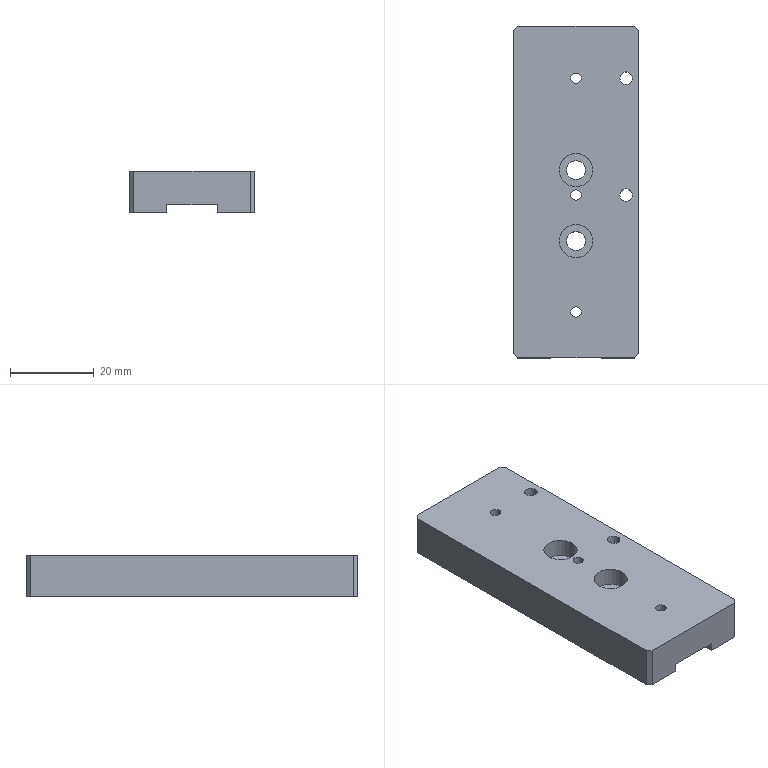Part | STEP file | 11-FG-E01911 | 1 solid | 34 faces | box 30 x 79.5 x 10 mm | volume 21106 mm3 | cylinder 18 | plane 16 | commonest cylinder face diameters 2.5 x6 3 x4 4.5 x4 8 x4
STEP:
#1=CARTESIAN_POINT('',(-4.,5.25,5.6));
#2=VERTEX_POINT('',#1);
#3=CARTESIAN_POINT('',(4.,5.25,5.6));
#4=VERTEX_POINT('',#3);
#5=CARTESIAN_POINT('',(0.,5.25,5.6));
#6=DIRECTION('',(0.,0.,1.));
#7=DIRECTION('',(1.,0.,0.));
#8=AXIS2_PLACEMENT_3D('',#5,#6,#7);
#9=CIRCLE('',#8,4.);
#10=EDGE_CURVE('',#2,#4,#9,.T.);
#11=ORIENTED_EDGE('',*,*,#10,.F.);
#12=CARTESIAN_POINT('',(-4.,5.25,10.));
#13=VERTEX_POINT('',#12);
#14=CARTESIAN_POINT('',(-4.,5.25,10.));
#15=DIRECTION('',(0.,0.,1.));
#16=VECTOR('',#15,1000.);
#17=LINE('',#14,#16);
#18=EDGE_CURVE('',#2,#13,#17,.T.);
#19=ORIENTED_EDGE('',*,*,#18,.T.);
#20=CARTESIAN_POINT('',(4.,5.25,10.));
#21=VERTEX_POINT('',#20);
#22=CARTESIAN_POINT('',(0.,5.25,10.));
#23=DIRECTION('',(0.,0.,1.));
#24=DIRECTION('',(1.,0.,0.));
#25=AXIS2_PLACEMENT_3D('',#22,#23,#24);
#26=CIRCLE('',#25,4.);
#27=EDGE_CURVE('',#13,#21,#26,.T.);
#28=ORIENTED_EDGE('',*,*,#27,.T.);
#29=CARTESIAN_POINT('',(4.,5.25,10.));
#30=DIRECTION('',(0.,0.,1.));
#31=VECTOR('',#30,1000.);
#32=LINE('',#29,#31);
#33=EDGE_CURVE('',#4,#21,#32,.T.);
#34=ORIENTED_EDGE('',*,*,#33,.F.);
#35=EDGE_LOOP('',(#11,#19,#28,#34));
#36=FACE_OUTER_BOUND('',#35,.T.);
#37=CARTESIAN_POINT('',(0.,5.25,10.));
#38=DIRECTION('',(0.,0.,1.));
#39=DIRECTION('',(1.,0.,0.));
#40=AXIS2_PLACEMENT_3D('',#37,#38,#39);
#41=CYLINDRICAL_SURFACE('',#40,4.);
#42=ADVANCED_FACE('',(#36),#41,.F.);
#43=CARTESIAN_POINT('',(2.25,5.25,2.));
#44=VERTEX_POINT('',#43);
#45=CARTESIAN_POINT('',(-2.25,5.25,2.));
#46=VERTEX_POINT('',#45);
#47=CARTESIAN_POINT('',(0.,5.25,2.));
#48=DIRECTION('',(0.,0.,-1.));
#49=DIRECTION('',(-1.,0.,0.));
#50=AXIS2_PLACEMENT_3D('',#47,#48,#49);
#51=CIRCLE('',#50,2.25);
#52=EDGE_CURVE('',#44,#46,#51,.T.);
#53=ORIENTED_EDGE('',*,*,#52,.T.);
#54=CARTESIAN_POINT('',(-2.25,5.25,5.6));
#55=VERTEX_POINT('',#54);
#56=CARTESIAN_POINT('',(-2.25,5.25,10.));
#57=DIRECTION('',(0.,0.,1.));
#58=VECTOR('',#57,1000.);
#59=LINE('',#56,#58);
#60=EDGE_CURVE('',#46,#55,#59,.T.);
#61=ORIENTED_EDGE('',*,*,#60,.T.);
#62=CARTESIAN_POINT('',(2.25,5.25,5.6));
#63=VERTEX_POINT('',#62);
#64=CARTESIAN_POINT('',(0.,5.25,5.6));
#65=DIRECTION('',(0.,0.,1.));
#66=DIRECTION('',(1.,0.,0.));
#67=AXIS2_PLACEMENT_3D('',#64,#65,#66);
#68=CIRCLE('',#67,2.25);
#69=EDGE_CURVE('',#55,#63,#68,.T.);
#70=ORIENTED_EDGE('',*,*,#69,.T.);
#71=CARTESIAN_POINT('',(2.25,5.25,10.));
#72=DIRECTION('',(0.,0.,1.));
#73=VECTOR('',#72,1000.);
#74=LINE('',#71,#73);
#75=EDGE_CURVE('',#44,#63,#74,.T.);
#76=ORIENTED_EDGE('',*,*,#75,.F.);
#77=EDGE_LOOP('',(#53,#61,#70,#76));
#78=FACE_OUTER_BOUND('',#77,.T.);
#79=CARTESIAN_POINT('',(0.,5.25,10.));
#80=DIRECTION('',(0.,0.,1.));
#81=DIRECTION('',(1.,0.,0.));
#82=AXIS2_PLACEMENT_3D('',#79,#80,#81);
#83=CYLINDRICAL_SURFACE('',#82,2.25);
#84=ADVANCED_FACE('',(#78),#83,.F.);
#85=CARTESIAN_POINT('',(-4.,-11.75,5.6));
#86=VERTEX_POINT('',#85);
#87=CARTESIAN_POINT('',(4.,-11.75,5.6));
#88=VERTEX_POINT('',#87);
#89=CARTESIAN_POINT('',(0.,-11.75,5.6));
#90=DIRECTION('',(0.,0.,1.));
#91=DIRECTION('',(1.,0.,0.));
#92=AXIS2_PLACEMENT_3D('',#89,#90,#91);
#93=CIRCLE('',#92,4.);
#94=EDGE_CURVE('',#86,#88,#93,.T.);
#95=ORIENTED_EDGE('',*,*,#94,.F.);
#96=CARTESIAN_POINT('',(-4.,-11.75,10.));
#97=VERTEX_POINT('',#96);
#98=CARTESIAN_POINT('',(-4.,-11.75,10.));
#99=DIRECTION('',(0.,0.,1.));
#100=VECTOR('',#99,1000.);
#101=LINE('',#98,#100);
#102=EDGE_CURVE('',#86,#97,#101,.T.);
#103=ORIENTED_EDGE('',*,*,#102,.T.);
#104=CARTESIAN_POINT('',(4.,-11.75,10.));
#105=VERTEX_POINT('',#104);
#106=CARTESIAN_POINT('',(0.,-11.75,10.));
#107=DIRECTION('',(0.,0.,1.));
#108=DIRECTION('',(1.,0.,0.));
#109=AXIS2_PLACEMENT_3D('',#106,#107,#108);
#110=CIRCLE('',#109,4.);
#111=EDGE_CURVE('',#97,#105,#110,.T.);
#112=ORIENTED_EDGE('',*,*,#111,.T.);
#113=CARTESIAN_POINT('',(4.,-11.75,10.));
#114=DIRECTION('',(0.,0.,1.));
#115=VECTOR('',#114,1000.);
#116=LINE('',#113,#115);
#117=EDGE_CURVE('',#88,#105,#116,.T.);
#118=ORIENTED_EDGE('',*,*,#117,.F.);
#119=EDGE_LOOP('',(#95,#103,#112,#118));
#120=FACE_OUTER_BOUND('',#119,.T.);
#121=CARTESIAN_POINT('',(0.,-11.75,10.));
#122=DIRECTION('',(0.,0.,1.));
#123=DIRECTION('',(1.,0.,0.));
#124=AXIS2_PLACEMENT_3D('',#121,#122,#123);
#125=CYLINDRICAL_SURFACE('',#124,4.);
#126=ADVANCED_FACE('',(#120),#125,.F.);
#127=CARTESIAN_POINT('',(2.25,-11.75,2.));
#128=VERTEX_POINT('',#127);
#129=CARTESIAN_POINT('',(-2.25,-11.75,2.));
#130=VERTEX_POINT('',#129);
#131=CARTESIAN_POINT('',(0.,-11.75,2.));
#132=DIRECTION('',(0.,0.,-1.));
#133=DIRECTION('',(-1.,0.,0.));
#134=AXIS2_PLACEMENT_3D('',#131,#132,#133);
#135=CIRCLE('',#134,2.25);
#136=EDGE_CURVE('',#128,#130,#135,.T.);
#137=ORIENTED_EDGE('',*,*,#136,.T.);
#138=CARTESIAN_POINT('',(-2.25,-11.75,5.6));
#139=VERTEX_POINT('',#138);
#140=CARTESIAN_POINT('',(-2.25,-11.75,10.));
#141=DIRECTION('',(0.,0.,1.));
#142=VECTOR('',#141,1000.);
#143=LINE('',#140,#142);
#144=EDGE_CURVE('',#130,#139,#143,.T.);
#145=ORIENTED_EDGE('',*,*,#144,.T.);
#146=CARTESIAN_POINT('',(2.25,-11.75,5.6));
#147=VERTEX_POINT('',#146);
#148=CARTESIAN_POINT('',(0.,-11.75,5.6));
#149=DIRECTION('',(0.,0.,1.));
#150=DIRECTION('',(1.,0.,0.));
#151=AXIS2_PLACEMENT_3D('',#148,#149,#150);
#152=CIRCLE('',#151,2.25);
#153=EDGE_CURVE('',#139,#147,#152,.T.);
#154=ORIENTED_EDGE('',*,*,#153,.T.);
#155=CARTESIAN_POINT('',(2.25,-11.75,10.));
#156=DIRECTION('',(0.,0.,1.));
#157=VECTOR('',#156,1000.);
#158=LINE('',#155,#157);
#159=EDGE_CURVE('',#128,#147,#158,.T.);
#160=ORIENTED_EDGE('',*,*,#159,.F.);
#161=EDGE_LOOP('',(#137,#145,#154,#160));
#162=FACE_OUTER_BOUND('',#161,.T.);
#163=CARTESIAN_POINT('',(0.,-11.75,10.));
#164=DIRECTION('',(0.,0.,1.));
#165=DIRECTION('',(1.,0.,0.));
#166=AXIS2_PLACEMENT_3D('',#163,#164,#165);
#167=CYLINDRICAL_SURFACE('',#166,2.25);
#168=ADVANCED_FACE('',(#162),#167,.F.);
#169=CARTESIAN_POINT('',(10.5,-0.75,0.));
#170=VERTEX_POINT('',#169);
#171=CARTESIAN_POINT('',(13.5,-0.75,0.));
#172=VERTEX_POINT('',#171);
#173=CARTESIAN_POINT('',(12.,-0.75,0.));
#174=DIRECTION('',(0.,0.,1.));
#175=DIRECTION('',(1.,0.,0.));
#176=AXIS2_PLACEMENT_3D('',#173,#174,#175);
#177=CIRCLE('',#176,1.5);
#178=EDGE_CURVE('',#170,#172,#177,.T.);
#179=ORIENTED_EDGE('',*,*,#178,.F.);
#180=CARTESIAN_POINT('',(10.5,-0.75,10.));
#181=VERTEX_POINT('',#180);
#182=CARTESIAN_POINT('',(10.5,-0.75,10.));
#183=DIRECTION('',(0.,0.,1.));
#184=VECTOR('',#183,1000.);
#185=LINE('',#182,#184);
#186=EDGE_CURVE('',#170,#181,#185,.T.);
#187=ORIENTED_EDGE('',*,*,#186,.T.);
#188=CARTESIAN_POINT('',(13.5,-0.75,10.));
#189=VERTEX_POINT('',#188);
#190=CARTESIAN_POINT('',(12.,-0.75,10.));
#191=DIRECTION('',(0.,0.,1.));
#192=DIRECTION('',(1.,0.,0.));
#193=AXIS2_PLACEMENT_3D('',#190,#191,#192);
#194=CIRCLE('',#193,1.5);
#195=EDGE_CURVE('',#181,#189,#194,.T.);
#196=ORIENTED_EDGE('',*,*,#195,.T.);
#197=CARTESIAN_POINT('',(13.5,-0.75,10.));
#198=DIRECTION('',(0.,0.,1.));
#199=VECTOR('',#198,1000.);
#200=LINE('',#197,#199);
#201=EDGE_CURVE('',#172,#189,#200,.T.);
#202=ORIENTED_EDGE('',*,*,#201,.F.);
#203=EDGE_LOOP('',(#179,#187,#196,#202));
#204=FACE_OUTER_BOUND('',#203,.T.);
#205=CARTESIAN_POINT('',(12.,-0.75,10.));
#206=DIRECTION('',(0.,0.,1.));
#207=DIRECTION('',(1.,0.,0.));
#208=AXIS2_PLACEMENT_3D('',#205,#206,#207);
#209=CYLINDRICAL_SURFACE('',#208,1.5);
#210=ADVANCED_FACE('',(#204),#209,.F.);
#211=CARTESIAN_POINT('',(10.5,27.25,0.));
#212=VERTEX_POINT('',#211);
#213=CARTESIAN_POINT('',(13.5,27.25,0.));
#214=VERTEX_POINT('',#213);
#215=CARTESIAN_POINT('',(12.,27.25,0.));
#216=DIRECTION('',(0.,0.,1.));
#217=DIRECTION('',(1.,0.,0.));
#218=AXIS2_PLACEMENT_3D('',#215,#216,#217);
#219=CIRCLE('',#218,1.5);
#220=EDGE_CURVE('',#212,#214,#219,.T.);
#221=ORIENTED_EDGE('',*,*,#220,.F.);
#222=CARTESIAN_POINT('',(10.5,27.25,10.));
#223=VERTEX_POINT('',#222);
#224=CARTESIAN_POINT('',(10.5,27.25,10.));
#225=DIRECTION('',(0.,0.,1.));
#226=VECTOR('',#225,1000.);
#227=LINE('',#224,#226);
#228=EDGE_CURVE('',#212,#223,#227,.T.);
#229=ORIENTED_EDGE('',*,*,#228,.T.);
#230=CARTESIAN_POINT('',(13.5,27.25,10.));
#231=VERTEX_POINT('',#230);
#232=CARTESIAN_POINT('',(12.,27.25,10.));
#233=DIRECTION('',(0.,0.,1.));
#234=DIRECTION('',(1.,0.,0.));
#235=AXIS2_PLACEMENT_3D('',#232,#233,#234);
#236=CIRCLE('',#235,1.5);
#237=EDGE_CURVE('',#223,#231,#236,.T.);
#238=ORIENTED_EDGE('',*,*,#237,.T.);
#239=CARTESIAN_POINT('',(13.5,27.25,10.));
#240=DIRECTION('',(0.,0.,1.));
#241=VECTOR('',#240,1000.);
#242=LINE('',#239,#241);
#243=EDGE_CURVE('',#214,#231,#242,.T.);
#244=ORIENTED_EDGE('',*,*,#243,.F.);
#245=EDGE_LOOP('',(#221,#229,#238,#244));
#246=FACE_OUTER_BOUND('',#245,.T.);
#247=CARTESIAN_POINT('',(12.,27.25,10.));
#248=DIRECTION('',(0.,0.,1.));
#249=DIRECTION('',(1.,0.,0.));
#250=AXIS2_PLACEMENT_3D('',#247,#248,#249);
#251=CYLINDRICAL_SURFACE('',#250,1.5);
#252=ADVANCED_FACE('',(#246),#251,.F.);
#253=CARTESIAN_POINT('',(1.25,-28.75,2.));
#254=VERTEX_POINT('',#253);
#255=CARTESIAN_POINT('',(-1.25,-28.75,2.));
#256=VERTEX_POINT('',#255);
#257=CARTESIAN_POINT('',(0.,-28.75,2.));
#258=DIRECTION('',(0.,0.,-1.));
#259=DIRECTION('',(-1.,0.,0.));
#260=AXIS2_PLACEMENT_3D('',#257,#258,#259);
#261=CIRCLE('',#260,1.25);
#262=EDGE_CURVE('',#254,#256,#261,.T.);
#263=ORIENTED_EDGE('',*,*,#262,.T.);
#264=CARTESIAN_POINT('',(-1.25,-28.75,10.));
#265=VERTEX_POINT('',#264);
#266=CARTESIAN_POINT('',(-1.25,-28.75,10.));
#267=DIRECTION('',(0.,0.,1.));
#268=VECTOR('',#267,1000.);
#269=LINE('',#266,#268);
#270=EDGE_CURVE('',#256,#265,#269,.T.);
#271=ORIENTED_EDGE('',*,*,#270,.T.);
#272=CARTESIAN_POINT('',(1.25,-28.75,10.));
#273=VERTEX_POINT('',#272);
#274=CARTESIAN_POINT('',(0.,-28.75,10.));
#275=DIRECTION('',(0.,0.,1.));
#276=DIRECTION('',(1.,0.,0.));
#277=AXIS2_PLACEMENT_3D('',#274,#275,#276);
#278=CIRCLE('',#277,1.25);
#279=EDGE_CURVE('',#265,#273,#278,.T.);
#280=ORIENTED_EDGE('',*,*,#279,.T.);
#281=CARTESIAN_POINT('',(1.25,-28.75,10.));
#282=DIRECTION('',(0.,0.,1.));
#283=VECTOR('',#282,1000.);
#284=LINE('',#281,#283);
#285=EDGE_CURVE('',#254,#273,#284,.T.);
#286=ORIENTED_EDGE('',*,*,#285,.F.);
#287=EDGE_LOOP('',(#263,#271,#280,#286));
#288=FACE_OUTER_BOUND('',#287,.T.);
#289=CARTESIAN_POINT('',(0.,-28.75,10.));
#290=DIRECTION('',(0.,0.,1.));
#291=DIRECTION('',(1.,0.,0.));
#292=AXIS2_PLACEMENT_3D('',#289,#290,#291);
#293=CYLINDRICAL_SURFACE('',#292,1.25);
#294=ADVANCED_FACE('',(#288),#293,.F.);
#295=CARTESIAN_POINT('',(1.25,-0.75,2.));
#296=VERTEX_POINT('',#295);
#297=CARTESIAN_POINT('',(-1.25,-0.75,2.));
#298=VERTEX_POINT('',#297);
#299=CARTESIAN_POINT('',(0.,-0.75,2.));
#300=DIRECTION('',(0.,0.,-1.));
#301=DIRECTION('',(-1.,0.,0.));
#302=AXIS2_PLACEMENT_3D('',#299,#300,#301);
#303=CIRCLE('',#302,1.25);
#304=EDGE_CURVE('',#296,#298,#303,.T.);
#305=ORIENTED_EDGE('',*,*,#304,.T.);
#306=CARTESIAN_POINT('',(-1.25,-0.75,10.));
#307=VERTEX_POINT('',#306);
#308=CARTESIAN_POINT('',(-1.25,-0.75,10.));
#309=DIRECTION('',(0.,0.,1.));
#310=VECTOR('',#309,1000.);
#311=LINE('',#308,#310);
#312=EDGE_CURVE('',#298,#307,#311,.T.);
#313=ORIENTED_EDGE('',*,*,#312,.T.);
#314=CARTESIAN_POINT('',(1.25,-0.75,10.));
#315=VERTEX_POINT('',#314);
#316=CARTESIAN_POINT('',(0.,-0.75,10.));
#317=DIRECTION('',(0.,0.,1.));
#318=DIRECTION('',(1.,0.,0.));
#319=AXIS2_PLACEMENT_3D('',#316,#317,#318);
#320=CIRCLE('',#319,1.25);
#321=EDGE_CURVE('',#307,#315,#320,.T.);
#322=ORIENTED_EDGE('',*,*,#321,.T.);
#323=CARTESIAN_POINT('',(1.25,-0.75,10.));
#324=DIRECTION('',(0.,0.,1.));
#325=VECTOR('',#324,1000.);
#326=LINE('',#323,#325);
#327=EDGE_CURVE('',#296,#315,#326,.T.);
#328=ORIENTED_EDGE('',*,*,#327,.F.);
#329=EDGE_LOOP('',(#305,#313,#322,#328));
#330=FACE_OUTER_BOUND('',#329,.T.);
#331=CARTESIAN_POINT('',(0.,-0.75,10.));
#332=DIRECTION('',(0.,0.,1.));
#333=DIRECTION('',(1.,0.,0.));
#334=AXIS2_PLACEMENT_3D('',#331,#332,#333);
#335=CYLINDRICAL_SURFACE('',#334,1.25);
#336=ADVANCED_FACE('',(#330),#335,.F.);
#337=CARTESIAN_POINT('',(1.25,27.25,2.));
#338=VERTEX_POINT('',#337);
#339=CARTESIAN_POINT('',(-1.25,27.25,2.));
#340=VERTEX_POINT('',#339);
#341=CARTESIAN_POINT('',(0.,27.25,2.));
#342=DIRECTION('',(0.,0.,-1.));
#343=DIRECTION('',(-1.,0.,0.));
#344=AXIS2_PLACEMENT_3D('',#341,#342,#343);
#345=CIRCLE('',#344,1.25);
#346=EDGE_CURVE('',#338,#340,#345,.T.);
#347=ORIENTED_EDGE('',*,*,#346,.T.);
#348=CARTESIAN_POINT('',(-1.25,27.25,10.));
#349=VERTEX_POINT('',#348);
#350=CARTESIAN_POINT('',(-1.25,27.25,10.));
#351=DIRECTION('',(0.,0.,1.));
#352=VECTOR('',#351,1000.);
#353=LINE('',#350,#352);
#354=EDGE_CURVE('',#340,#349,#353,.T.);
#355=ORIENTED_EDGE('',*,*,#354,.T.);
#356=CARTESIAN_POINT('',(1.25,27.25,10.));
#357=VERTEX_POINT('',#356);
#358=CARTESIAN_POINT('',(0.,27.25,10.));
#359=DIRECTION('',(0.,0.,1.));
#360=DIRECTION('',(1.,0.,0.));
#361=AXIS2_PLACEMENT_3D('',#358,#359,#360);
#362=CIRCLE('',#361,1.25);
#363=EDGE_CURVE('',#349,#357,#362,.T.);
#364=ORIENTED_EDGE('',*,*,#363,.T.);
#365=CARTESIAN_POINT('',(1.25,27.25,10.));
#366=DIRECTION('',(0.,0.,1.));
#367=VECTOR('',#366,1000.);
#368=LINE('',#365,#367);
#369=EDGE_CURVE('',#338,#357,#368,.T.);
#370=ORIENTED_EDGE('',*,*,#369,.F.);
#371=EDGE_LOOP('',(#347,#355,#364,#370));
#372=FACE_OUTER_BOUND('',#371,.T.);
#373=CARTESIAN_POINT('',(0.,27.25,10.));
#374=DIRECTION('',(0.,0.,1.));
#375=DIRECTION('',(1.,0.,0.));
#376=AXIS2_PLACEMENT_3D('',#373,#374,#375);
#377=CYLINDRICAL_SURFACE('',#376,1.25);
#378=ADVANCED_FACE('',(#372),#377,.F.);
#379=CARTESIAN_POINT('',(12.,-0.75,0.));
#380=DIRECTION('',(0.,0.,1.));
#381=DIRECTION('',(1.,0.,0.));
#382=AXIS2_PLACEMENT_3D('',#379,#380,#381);
#383=CIRCLE('',#382,1.5);
#384=EDGE_CURVE('',#172,#170,#383,.T.);
#385=ORIENTED_EDGE('',*,*,#384,.T.);
#386=ORIENTED_EDGE('',*,*,#178,.T.);
#387=EDGE_LOOP('',(#385,#386));
#388=FACE_BOUND('',#387,.T.);
#389=CARTESIAN_POINT('',(12.,27.25,0.));
#390=DIRECTION('',(0.,0.,1.));
#391=DIRECTION('',(1.,0.,0.));
#392=AXIS2_PLACEMENT_3D('',#389,#390,#391);
#393=CIRCLE('',#392,1.5);
#394=EDGE_CURVE('',#214,#212,#393,.T.);
#395=ORIENTED_EDGE('',*,*,#394,.T.);
#396=ORIENTED_EDGE('',*,*,#220,.T.);
#397=EDGE_LOOP('',(#395,#396));
#398=FACE_BOUND('',#397,.T.);
#399=CARTESIAN_POINT('',(15.,-38.75,0.));
#400=VERTEX_POINT('',#399);
#401=CARTESIAN_POINT('',(15.,38.75,0.));
#402=VERTEX_POINT('',#401);
#403=CARTESIAN_POINT('',(15.,-39.75,0.));
#404=DIRECTION('',(0.,1.,0.));
#405=VECTOR('',#404,1000.);
#406=LINE('',#403,#405);
#407=EDGE_CURVE('',#400,#402,#406,.T.);
#408=ORIENTED_EDGE('',*,*,#407,.F.);
#409=CARTESIAN_POINT('',(14.,-39.75,0.));
#410=VERTEX_POINT('',#409);
#411=CARTESIAN_POINT('',(26.875,-26.875,0.));
#412=DIRECTION('',(-0.7071,-0.7071,0.));
#413=VECTOR('',#412,1000.);
#414=LINE('',#411,#413);
#415=EDGE_CURVE('',#400,#410,#414,.T.);
#416=ORIENTED_EDGE('',*,*,#415,.T.);
#417=CARTESIAN_POINT('',(6.,-39.75,0.));
#418=VERTEX_POINT('',#417);
#419=CARTESIAN_POINT('',(-15.,-39.75,0.));
#420=DIRECTION('',(1.,0.,0.));
#421=VECTOR('',#420,1000.);
#422=LINE('',#419,#421);
#423=EDGE_CURVE('',#418,#410,#422,.T.);
#424=ORIENTED_EDGE('',*,*,#423,.F.);
#425=CARTESIAN_POINT('',(6.,39.75,0.));
#426=VERTEX_POINT('',#425);
#427=CARTESIAN_POINT('',(6.,-39.75,0.));
#428=DIRECTION('',(0.,-1.,0.));
#429=VECTOR('',#428,1000.);
#430=LINE('',#427,#429);
#431=EDGE_CURVE('',#426,#418,#430,.T.);
#432=ORIENTED_EDGE('',*,*,#431,.F.);
#433=CARTESIAN_POINT('',(14.,39.75,0.));
#434=VERTEX_POINT('',#433);
#435=CARTESIAN_POINT('',(-15.,39.75,0.));
#436=DIRECTION('',(-1.,0.,0.));
#437=VECTOR('',#436,1000.);
#438=LINE('',#435,#437);
#439=EDGE_CURVE('',#434,#426,#438,.T.);
#440=ORIENTED_EDGE('',*,*,#439,.F.);
#441=CARTESIAN_POINT('',(26.875,26.875,0.));
#442=DIRECTION('',(0.7071,-0.7071,0.));
#443=VECTOR('',#442,1000.);
#444=LINE('',#441,#443);
#445=EDGE_CURVE('',#434,#402,#444,.T.);
#446=ORIENTED_EDGE('',*,*,#445,.T.);
#447=EDGE_LOOP('',(#408,#416,#424,#432,#440,#446));
#448=FACE_OUTER_BOUND('',#447,.T.);
#449=CARTESIAN_POINT('',(0.,0.,0.));
#450=DIRECTION('',(0.,0.,-1.));
#451=DIRECTION('',(-1.,0.,0.));
#452=AXIS2_PLACEMENT_3D('',#449,#450,#451);
#453=PLANE('',#452);
#454=ADVANCED_FACE('',(#388,#398,#448),#453,.T.);
#455=CARTESIAN_POINT('',(15.,-38.75,10.));
#456=VERTEX_POINT('',#455);
#457=CARTESIAN_POINT('',(15.,38.75,10.));
#458=VERTEX_POINT('',#457);
#459=CARTESIAN_POINT('',(15.,-39.75,10.));
#460=DIRECTION('',(0.,1.,0.));
#461=VECTOR('',#460,1000.);
#462=LINE('',#459,#461);
#463=EDGE_CURVE('',#456,#458,#462,.T.);
#464=ORIENTED_EDGE('',*,*,#463,.F.);
#465=CARTESIAN_POINT('',(15.,-38.75,10.));
#466=DIRECTION('',(0.,0.,-1.));
#467=VECTOR('',#466,1000.);
#468=LINE('',#465,#467);
#469=EDGE_CURVE('',#456,#400,#468,.T.);
#470=ORIENTED_EDGE('',*,*,#469,.T.);
#471=ORIENTED_EDGE('',*,*,#407,.T.);
#472=CARTESIAN_POINT('',(15.,38.75,10.));
#473=DIRECTION('',(0.,0.,1.));
#474=VECTOR('',#473,1000.);
#475=LINE('',#472,#474);
#476=EDGE_CURVE('',#402,#458,#475,.T.);
#477=ORIENTED_EDGE('',*,*,#476,.T.);
#478=EDGE_LOOP('',(#464,#470,#471,#477));
#479=FACE_OUTER_BOUND('',#478,.T.);
#480=CARTESIAN_POINT('',(15.,-39.75,10.));
#481=DIRECTION('',(-1.,0.,0.));
#482=DIRECTION('',(0.,0.,1.));
#483=AXIS2_PLACEMENT_3D('',#480,#481,#482);
#484=PLANE('',#483);
#485=ADVANCED_FACE('',(#479),#484,.F.);
#486=CARTESIAN_POINT('',(14.,39.75,10.));
#487=VERTEX_POINT('',#486);
#488=CARTESIAN_POINT('',(-14.,39.75,10.));
#489=VERTEX_POINT('',#488);
#490=CARTESIAN_POINT('',(-15.,39.75,10.));
#491=DIRECTION('',(-1.,0.,0.));
#492=VECTOR('',#491,1000.);
#493=LINE('',#490,#492);
#494=EDGE_CURVE('',#487,#489,#493,.T.);
#495=ORIENTED_EDGE('',*,*,#494,.F.);
#496=CARTESIAN_POINT('',(14.,39.75,10.));
#497=DIRECTION('',(0.,0.,-1.));
#498=VECTOR('',#497,1000.);
#499=LINE('',#496,#498);
#500=EDGE_CURVE('',#487,#434,#499,.T.);
#501=ORIENTED_EDGE('',*,*,#500,.T.);
#502=ORIENTED_EDGE('',*,*,#439,.T.);
#503=CARTESIAN_POINT('',(6.,39.75,2.));
#504=VERTEX_POINT('',#503);
#505=CARTESIAN_POINT('',(6.,39.75,2.));
#506=DIRECTION('',(0.,0.,-1.));
#507=VECTOR('',#506,1000.);
#508=LINE('',#505,#507);
#509=EDGE_CURVE('',#504,#426,#508,.T.);
#510=ORIENTED_EDGE('',*,*,#509,.F.);
#511=CARTESIAN_POINT('',(-6.,39.75,2.));
#512=VERTEX_POINT('',#511);
#513=CARTESIAN_POINT('',(-6.,39.75,2.));
#514=DIRECTION('',(1.,0.,0.));
#515=VECTOR('',#514,1000.);
#516=LINE('',#513,#515);
#517=EDGE_CURVE('',#512,#504,#516,.T.);
#518=ORIENTED_EDGE('',*,*,#517,.F.);
#519=CARTESIAN_POINT('',(-6.,39.75,0.));
#520=VERTEX_POINT('',#519);
#521=CARTESIAN_POINT('',(-6.,39.75,2.));
#522=DIRECTION('',(0.,0.,-1.));
#523=VECTOR('',#522,1000.);
#524=LINE('',#521,#523);
#525=EDGE_CURVE('',#512,#520,#524,.T.);
#526=ORIENTED_EDGE('',*,*,#525,.T.);
#527=CARTESIAN_POINT('',(-14.,39.75,0.));
#528=VERTEX_POINT('',#527);
#529=CARTESIAN_POINT('',(-15.,39.75,0.));
#530=DIRECTION('',(-1.,0.,0.));
#531=VECTOR('',#530,1000.);
#532=LINE('',#529,#531);
#533=EDGE_CURVE('',#520,#528,#532,.T.);
#534=ORIENTED_EDGE('',*,*,#533,.T.);
#535=CARTESIAN_POINT('',(-14.,39.75,10.));
#536=DIRECTION('',(0.,0.,1.));
#537=VECTOR('',#536,1000.);
#538=LINE('',#535,#537);
#539=EDGE_CURVE('',#528,#489,#538,.T.);
#540=ORIENTED_EDGE('',*,*,#539,.T.);
#541=EDGE_LOOP('',(#495,#501,#502,#510,#518,#526,#534,#540));
#542=FACE_OUTER_BOUND('',#541,.T.);
#543=CARTESIAN_POINT('',(-15.,39.75,10.));
#544=DIRECTION('',(0.,-1.,0.));
#545=DIRECTION('',(0.,0.,-1.));
#546=AXIS2_PLACEMENT_3D('',#543,#544,#545);
#547=PLANE('',#546);
#548=ADVANCED_FACE('',(#542),#547,.F.);
#549=CARTESIAN_POINT('',(-15.,38.75,0.));
#550=VERTEX_POINT('',#549);
#551=CARTESIAN_POINT('',(-15.,-38.75,0.));
#552=VERTEX_POINT('',#551);
#553=CARTESIAN_POINT('',(-15.,-39.75,0.));
#554=DIRECTION('',(0.,-1.,0.));
#555=VECTOR('',#554,1000.);
#556=LINE('',#553,#555);
#557=EDGE_CURVE('',#550,#552,#556,.T.);
#558=ORIENTED_EDGE('',*,*,#557,.T.);
#559=CARTESIAN_POINT('',(-15.,-38.75,10.));
#560=VERTEX_POINT('',#559);
#561=CARTESIAN_POINT('',(-15.,-38.75,10.));
#562=DIRECTION('',(0.,0.,1.));
#563=VECTOR('',#562,1000.);
#564=LINE('',#561,#563);
#565=EDGE_CURVE('',#552,#560,#564,.T.);
#566=ORIENTED_EDGE('',*,*,#565,.T.);
#567=CARTESIAN_POINT('',(-15.,38.75,10.));
#568=VERTEX_POINT('',#567);
#569=CARTESIAN_POINT('',(-15.,-39.75,10.));
#570=DIRECTION('',(0.,-1.,0.));
#571=VECTOR('',#570,1000.);
#572=LINE('',#569,#571);
#573=EDGE_CURVE('',#568,#560,#572,.T.);
#574=ORIENTED_EDGE('',*,*,#573,.F.);
#575=CARTESIAN_POINT('',(-15.,38.75,10.));
#576=DIRECTION('',(0.,0.,-1.));
#577=VECTOR('',#576,1000.);
#578=LINE('',#575,#577);
#579=EDGE_CURVE('',#568,#550,#578,.T.);
#580=ORIENTED_EDGE('',*,*,#579,.T.);
#581=EDGE_LOOP('',(#558,#566,#574,#580));
#582=FACE_OUTER_BOUND('',#581,.T.);
#583=CARTESIAN_POINT('',(-15.,-39.75,10.));
#584=DIRECTION('',(1.,0.,0.));
#585=DIRECTION('',(0.,0.,-1.));
#586=AXIS2_PLACEMENT_3D('',#583,#584,#585);
#587=PLANE('',#586);
#588=ADVANCED_FACE('',(#582),#587,.F.);
#589=CARTESIAN_POINT('',(-14.,-39.75,10.));
#590=VERTEX_POINT('',#589);
#591=CARTESIAN_POINT('',(14.,-39.75,10.));
#592=VERTEX_POINT('',#591);
#593=CARTESIAN_POINT('',(-15.,-39.75,10.));
#594=DIRECTION('',(1.,0.,0.));
#595=VECTOR('',#594,1000.);
#596=LINE('',#593,#595);
#597=EDGE_CURVE('',#590,#592,#596,.T.);
#598=ORIENTED_EDGE('',*,*,#597,.F.);
#599=CARTESIAN_POINT('',(-14.,-39.75,0.));
#600=VERTEX_POINT('',#599);
#601=CARTESIAN_POINT('',(-14.,-39.75,10.));
#602=DIRECTION('',(0.,0.,-1.));
#603=VECTOR('',#602,1000.);
#604=LINE('',#601,#603);
#605=EDGE_CURVE('',#590,#600,#604,.T.);
#606=ORIENTED_EDGE('',*,*,#605,.T.);
#607=CARTESIAN_POINT('',(-6.,-39.75,0.));
#608=VERTEX_POINT('',#607);
#609=CARTESIAN_POINT('',(-15.,-39.75,0.));
#610=DIRECTION('',(1.,0.,0.));
#611=VECTOR('',#610,1000.);
#612=LINE('',#609,#611);
#613=EDGE_CURVE('',#600,#608,#612,.T.);
#614=ORIENTED_EDGE('',*,*,#613,.T.);
#615=CARTESIAN_POINT('',(-6.,-39.75,2.));
#616=VERTEX_POINT('',#615);
#617=CARTESIAN_POINT('',(-6.,-39.75,2.));
#618=DIRECTION('',(0.,0.,-1.));
#619=VECTOR('',#618,1000.);
#620=LINE('',#617,#619);
#621=EDGE_CURVE('',#616,#608,#620,.T.);
#622=ORIENTED_EDGE('',*,*,#621,.F.);
#623=CARTESIAN_POINT('',(6.,-39.75,2.));
#624=VERTEX_POINT('',#623);
#625=CARTESIAN_POINT('',(-6.,-39.75,2.));
#626=DIRECTION('',(-1.,0.,0.));
#627=VECTOR('',#626,1000.);
#628=LINE('',#625,#627);
#629=EDGE_CURVE('',#624,#616,#628,.T.);
#630=ORIENTED_EDGE('',*,*,#629,.F.);
#631=CARTESIAN_POINT('',(6.,-39.75,2.));
#632=DIRECTION('',(0.,0.,-1.));
#633=VECTOR('',#632,1000.);
#634=LINE('',#631,#633);
#635=EDGE_CURVE('',#624,#418,#634,.T.);
#636=ORIENTED_EDGE('',*,*,#635,.T.);
#637=ORIENTED_EDGE('',*,*,#423,.T.);
#638=CARTESIAN_POINT('',(14.,-39.75,10.));
#639=DIRECTION('',(0.,0.,1.));
#640=VECTOR('',#639,1000.);
#641=LINE('',#638,#640);
#642=EDGE_CURVE('',#410,#592,#641,.T.);
#643=ORIENTED_EDGE('',*,*,#642,.T.);
#644=EDGE_LOOP('',(#598,#606,#614,#622,#630,#636,#637,#643));
#645=FACE_OUTER_BOUND('',#644,.T.);
#646=CARTESIAN_POINT('',(-15.,-39.75,10.));
#647=DIRECTION('',(0.,1.,0.));
#648=DIRECTION('',(0.,0.,1.));
#649=AXIS2_PLACEMENT_3D('',#646,#647,#648);
#650=PLANE('',#649);
#651=ADVANCED_FACE('',(#645),#650,.F.);
#652=CARTESIAN_POINT('',(0.,5.25,10.));
#653=DIRECTION('',(0.,0.,1.));
#654=DIRECTION('',(1.,0.,0.));
#655=AXIS2_PLACEMENT_3D('',#652,#653,#654);
#656=CIRCLE('',#655,4.);
#657=EDGE_CURVE('',#21,#13,#656,.T.);
#658=ORIENTED_EDGE('',*,*,#657,.F.);
#659=ORIENTED_EDGE('',*,*,#27,.F.);
#660=EDGE_LOOP('',(#658,#659));
#661=FACE_BOUND('',#660,.T.);
#662=CARTESIAN_POINT('',(0.,-11.75,10.));
#663=DIRECTION('',(0.,0.,1.));
#664=DIRECTION('',(1.,0.,0.));
#665=AXIS2_PLACEMENT_3D('',#662,#663,#664);
#666=CIRCLE('',#665,4.);
#667=EDGE_CURVE('',#105,#97,#666,.T.);
#668=ORIENTED_EDGE('',*,*,#667,.F.);
#669=ORIENTED_EDGE('',*,*,#111,.F.);
#670=EDGE_LOOP('',(#668,#669));
#671=FACE_BOUND('',#670,.T.);
#672=CARTESIAN_POINT('',(12.,-0.75,10.));
#673=DIRECTION('',(0.,0.,1.));
#674=DIRECTION('',(1.,0.,0.));
#675=AXIS2_PLACEMENT_3D('',#672,#673,#674);
#676=CIRCLE('',#675,1.5);
#677=EDGE_CURVE('',#189,#181,#676,.T.);
#678=ORIENTED_EDGE('',*,*,#677,.F.);
#679=ORIENTED_EDGE('',*,*,#195,.F.);
#680=EDGE_LOOP('',(#678,#679));
#681=FACE_BOUND('',#680,.T.);
#682=CARTESIAN_POINT('',(12.,27.25,10.));
#683=DIRECTION('',(0.,0.,1.));
#684=DIRECTION('',(1.,0.,0.));
#685=AXIS2_PLACEMENT_3D('',#682,#683,#684);
#686=CIRCLE('',#685,1.5);
#687=EDGE_CURVE('',#231,#223,#686,.T.);
#688=ORIENTED_EDGE('',*,*,#687,.F.);
#689=ORIENTED_EDGE('',*,*,#237,.F.);
#690=EDGE_LOOP('',(#688,#689));
#691=FACE_BOUND('',#690,.T.);
#692=CARTESIAN_POINT('',(0.,-28.75,10.));
#693=DIRECTION('',(0.,0.,1.));
#694=DIRECTION('',(1.,0.,0.));
#695=AXIS2_PLACEMENT_3D('',#692,#693,#694);
#696=CIRCLE('',#695,1.25);
#697=EDGE_CURVE('',#273,#265,#696,.T.);
#698=ORIENTED_EDGE('',*,*,#697,.F.);
#699=ORIENTED_EDGE('',*,*,#279,.F.);
#700=EDGE_LOOP('',(#698,#699));
#701=FACE_BOUND('',#700,.T.);
#702=CARTESIAN_POINT('',(0.,-0.75,10.));
#703=DIRECTION('',(0.,0.,1.));
#704=DIRECTION('',(1.,0.,0.));
#705=AXIS2_PLACEMENT_3D('',#702,#703,#704);
#706=CIRCLE('',#705,1.25);
#707=EDGE_CURVE('',#315,#307,#706,.T.);
#708=ORIENTED_EDGE('',*,*,#707,.F.);
#709=ORIENTED_EDGE('',*,*,#321,.F.);
#710=EDGE_LOOP('',(#708,#709));
#711=FACE_BOUND('',#710,.T.);
#712=CARTESIAN_POINT('',(0.,27.25,10.));
#713=DIRECTION('',(0.,0.,1.));
#714=DIRECTION('',(1.,0.,0.));
#715=AXIS2_PLACEMENT_3D('',#712,#713,#714);
#716=CIRCLE('',#715,1.25);
#717=EDGE_CURVE('',#357,#349,#716,.T.);
#718=ORIENTED_EDGE('',*,*,#717,.F.);
#719=ORIENTED_EDGE('',*,*,#363,.F.);
#720=EDGE_LOOP('',(#718,#719));
#721=FACE_BOUND('',#720,.T.);
#722=ORIENTED_EDGE('',*,*,#573,.T.);
#723=CARTESIAN_POINT('',(-14.,-39.75,10.));
#724=DIRECTION('',(0.7071,-0.7071,0.));
#725=VECTOR('',#724,1000.);
#726=LINE('',#723,#725);
#727=EDGE_CURVE('',#560,#590,#726,.T.);
#728=ORIENTED_EDGE('',*,*,#727,.T.);
#729=ORIENTED_EDGE('',*,*,#597,.T.);
#730=CARTESIAN_POINT('',(15.,-38.75,10.));
#731=DIRECTION('',(0.7071,0.7071,0.));
#732=VECTOR('',#731,1000.);
#733=LINE('',#730,#732);
#734=EDGE_CURVE('',#592,#456,#733,.T.);
#735=ORIENTED_EDGE('',*,*,#734,.T.);
#736=ORIENTED_EDGE('',*,*,#463,.T.);
#737=CARTESIAN_POINT('',(14.,39.75,10.));
#738=DIRECTION('',(-0.7071,0.7071,0.));
#739=VECTOR('',#738,1000.);
#740=LINE('',#737,#739);
#741=EDGE_CURVE('',#458,#487,#740,.T.);
#742=ORIENTED_EDGE('',*,*,#741,.T.);
#743=ORIENTED_EDGE('',*,*,#494,.T.);
#744=CARTESIAN_POINT('',(-15.,38.75,10.));
#745=DIRECTION('',(-0.7071,-0.7071,0.));
#746=VECTOR('',#745,1000.);
#747=LINE('',#744,#746);
#748=EDGE_CURVE('',#489,#568,#747,.T.);
#749=ORIENTED_EDGE('',*,*,#748,.T.);
#750=EDGE_LOOP('',(#722,#728,#729,#735,#736,#742,#743,#749));
#751=FACE_OUTER_BOUND('',#750,.T.);
#752=CARTESIAN_POINT('',(0.,0.,10.));
#753=DIRECTION('',(0.,0.,-1.));
#754=DIRECTION('',(-1.,0.,0.));
#755=AXIS2_PLACEMENT_3D('',#752,#753,#754);
#756=PLANE('',#755);
#757=ADVANCED_FACE('',(#661,#671,#681,#691,#701,#711,#721,#751),#756,.F.);
#758=ORIENTED_EDGE('',*,*,#613,.F.);
#759=CARTESIAN_POINT('',(-26.875,-26.875,0.));
#760=DIRECTION('',(-0.7071,0.7071,0.));
#761=VECTOR('',#760,1000.);
#762=LINE('',#759,#761);
#763=EDGE_CURVE('',#600,#552,#762,.T.);
#764=ORIENTED_EDGE('',*,*,#763,.T.);
#765=ORIENTED_EDGE('',*,*,#557,.F.);
#766=CARTESIAN_POINT('',(-26.875,26.875,0.));
#767=DIRECTION('',(0.7071,0.7071,0.));
#768=VECTOR('',#767,1000.);
#769=LINE('',#766,#768);
#770=EDGE_CURVE('',#550,#528,#769,.T.);
#771=ORIENTED_EDGE('',*,*,#770,.T.);
#772=ORIENTED_EDGE('',*,*,#533,.F.);
#773=CARTESIAN_POINT('',(-6.,-39.75,0.));
#774=DIRECTION('',(0.,1.,0.));
#775=VECTOR('',#774,1000.);
#776=LINE('',#773,#775);
#777=EDGE_CURVE('',#608,#520,#776,.T.);
#778=ORIENTED_EDGE('',*,*,#777,.F.);
#779=EDGE_LOOP('',(#758,#764,#765,#771,#772,#778));
#780=FACE_OUTER_BOUND('',#779,.T.);
#781=CARTESIAN_POINT('',(0.,0.,0.));
#782=DIRECTION('',(0.,0.,-1.));
#783=DIRECTION('',(-1.,0.,0.));
#784=AXIS2_PLACEMENT_3D('',#781,#782,#783);
#785=PLANE('',#784);
#786=ADVANCED_FACE('',(#780),#785,.T.);
#787=ORIENTED_EDGE('',*,*,#431,.T.);
#788=ORIENTED_EDGE('',*,*,#635,.F.);
#789=CARTESIAN_POINT('',(6.,-39.75,2.));
#790=DIRECTION('',(0.,-1.,0.));
#791=VECTOR('',#790,1000.);
#792=LINE('',#789,#791);
#793=EDGE_CURVE('',#504,#624,#792,.T.);
#794=ORIENTED_EDGE('',*,*,#793,.F.);
#795=ORIENTED_EDGE('',*,*,#509,.T.);
#796=EDGE_LOOP('',(#787,#788,#794,#795));
#797=FACE_OUTER_BOUND('',#796,.T.);
#798=CARTESIAN_POINT('',(6.,-39.75,2.));
#799=DIRECTION('',(1.,0.,0.));
#800=DIRECTION('',(0.,0.,-1.));
#801=AXIS2_PLACEMENT_3D('',#798,#799,#800);
#802=PLANE('',#801);
#803=ADVANCED_FACE('',(#797),#802,.F.);
#804=ORIENTED_EDGE('',*,*,#777,.T.);
#805=ORIENTED_EDGE('',*,*,#525,.F.);
#806=CARTESIAN_POINT('',(-6.,-39.75,2.));
#807=DIRECTION('',(0.,1.,0.));
#808=VECTOR('',#807,1000.);
#809=LINE('',#806,#808);
#810=EDGE_CURVE('',#616,#512,#809,.T.);
#811=ORIENTED_EDGE('',*,*,#810,.F.);
#812=ORIENTED_EDGE('',*,*,#621,.T.);
#813=EDGE_LOOP('',(#804,#805,#811,#812));
#814=FACE_OUTER_BOUND('',#813,.T.);
#815=CARTESIAN_POINT('',(-6.,-39.75,2.));
#816=DIRECTION('',(-1.,0.,0.));
#817=DIRECTION('',(0.,0.,1.));
#818=AXIS2_PLACEMENT_3D('',#815,#816,#817);
#819=PLANE('',#818);
#820=ADVANCED_FACE('',(#814),#819,.F.);
#821=ORIENTED_EDGE('',*,*,#52,.F.);
#822=CARTESIAN_POINT('',(0.,5.25,2.));
#823=DIRECTION('',(0.,0.,-1.));
#824=DIRECTION('',(-1.,0.,0.));
#825=AXIS2_PLACEMENT_3D('',#822,#823,#824);
#826=CIRCLE('',#825,2.25);
#827=EDGE_CURVE('',#46,#44,#826,.T.);
#828=ORIENTED_EDGE('',*,*,#827,.F.);
#829=EDGE_LOOP('',(#821,#828));
#830=FACE_BOUND('',#829,.T.);
#831=ORIENTED_EDGE('',*,*,#136,.F.);
#832=CARTESIAN_POINT('',(0.,-11.75,2.));
#833=DIRECTION('',(0.,0.,-1.));
#834=DIRECTION('',(-1.,0.,0.));
#835=AXIS2_PLACEMENT_3D('',#832,#833,#834);
#836=CIRCLE('',#835,2.25);
#837=EDGE_CURVE('',#130,#128,#836,.T.);
#838=ORIENTED_EDGE('',*,*,#837,.F.);
#839=EDGE_LOOP('',(#831,#838));
#840=FACE_BOUND('',#839,.T.);
#841=ORIENTED_EDGE('',*,*,#262,.F.);
#842=CARTESIAN_POINT('',(0.,-28.75,2.));
#843=DIRECTION('',(0.,0.,-1.));
#844=DIRECTION('',(-1.,0.,0.));
#845=AXIS2_PLACEMENT_3D('',#842,#843,#844);
#846=CIRCLE('',#845,1.25);
#847=EDGE_CURVE('',#256,#254,#846,.T.);
#848=ORIENTED_EDGE('',*,*,#847,.F.);
#849=EDGE_LOOP('',(#841,#848));
#850=FACE_BOUND('',#849,.T.);
#851=ORIENTED_EDGE('',*,*,#304,.F.);
#852=CARTESIAN_POINT('',(0.,-0.75,2.));
#853=DIRECTION('',(0.,0.,-1.));
#854=DIRECTION('',(-1.,0.,0.));
#855=AXIS2_PLACEMENT_3D('',#852,#853,#854);
#856=CIRCLE('',#855,1.25);
#857=EDGE_CURVE('',#298,#296,#856,.T.);
#858=ORIENTED_EDGE('',*,*,#857,.F.);
#859=EDGE_LOOP('',(#851,#858));
#860=FACE_BOUND('',#859,.T.);
#861=ORIENTED_EDGE('',*,*,#346,.F.);
#862=CARTESIAN_POINT('',(0.,27.25,2.));
#863=DIRECTION('',(0.,0.,-1.));
#864=DIRECTION('',(-1.,0.,0.));
#865=AXIS2_PLACEMENT_3D('',#862,#863,#864);
#866=CIRCLE('',#865,1.25);
#867=EDGE_CURVE('',#340,#338,#866,.T.);
#868=ORIENTED_EDGE('',*,*,#867,.F.);
#869=EDGE_LOOP('',(#861,#868));
#870=FACE_BOUND('',#869,.T.);
#871=ORIENTED_EDGE('',*,*,#793,.T.);
#872=ORIENTED_EDGE('',*,*,#629,.T.);
#873=ORIENTED_EDGE('',*,*,#810,.T.);
#874=ORIENTED_EDGE('',*,*,#517,.T.);
#875=EDGE_LOOP('',(#871,#872,#873,#874));
#876=FACE_OUTER_BOUND('',#875,.T.);
#877=CARTESIAN_POINT('',(0.,0.,2.));
#878=DIRECTION('',(0.,0.,-1.));
#879=DIRECTION('',(-1.,0.,0.));
#880=AXIS2_PLACEMENT_3D('',#877,#878,#879);
#881=PLANE('',#880);
#882=ADVANCED_FACE('',(#830,#840,#850,#860,#870,#876),#881,.T.);
#883=ORIENTED_EDGE('',*,*,#354,.F.);
#884=ORIENTED_EDGE('',*,*,#867,.T.);
#885=ORIENTED_EDGE('',*,*,#369,.T.);
#886=ORIENTED_EDGE('',*,*,#717,.T.);
#887=EDGE_LOOP('',(#883,#884,#885,#886));
#888=FACE_OUTER_BOUND('',#887,.T.);
#889=CARTESIAN_POINT('',(0.,27.25,10.));
#890=DIRECTION('',(0.,0.,1.));
#891=DIRECTION('',(1.,0.,0.));
#892=AXIS2_PLACEMENT_3D('',#889,#890,#891);
#893=CYLINDRICAL_SURFACE('',#892,1.25);
#894=ADVANCED_FACE('',(#888),#893,.F.);
#895=ORIENTED_EDGE('',*,*,#312,.F.);
#896=ORIENTED_EDGE('',*,*,#857,.T.);
#897=ORIENTED_EDGE('',*,*,#327,.T.);
#898=ORIENTED_EDGE('',*,*,#707,.T.);
#899=EDGE_LOOP('',(#895,#896,#897,#898));
#900=FACE_OUTER_BOUND('',#899,.T.);
#901=CARTESIAN_POINT('',(0.,-0.75,10.));
#902=DIRECTION('',(0.,0.,1.));
#903=DIRECTION('',(1.,0.,0.));
#904=AXIS2_PLACEMENT_3D('',#901,#902,#903);
#905=CYLINDRICAL_SURFACE('',#904,1.25);
#906=ADVANCED_FACE('',(#900),#905,.F.);
#907=ORIENTED_EDGE('',*,*,#270,.F.);
#908=ORIENTED_EDGE('',*,*,#847,.T.);
#909=ORIENTED_EDGE('',*,*,#285,.T.);
#910=ORIENTED_EDGE('',*,*,#697,.T.);
#911=EDGE_LOOP('',(#907,#908,#909,#910));
#912=FACE_OUTER_BOUND('',#911,.T.);
#913=CARTESIAN_POINT('',(0.,-28.75,10.));
#914=DIRECTION('',(0.,0.,1.));
#915=DIRECTION('',(1.,0.,0.));
#916=AXIS2_PLACEMENT_3D('',#913,#914,#915);
#917=CYLINDRICAL_SURFACE('',#916,1.25);
#918=ADVANCED_FACE('',(#912),#917,.F.);
#919=ORIENTED_EDGE('',*,*,#228,.F.);
#920=ORIENTED_EDGE('',*,*,#394,.F.);
#921=ORIENTED_EDGE('',*,*,#243,.T.);
#922=ORIENTED_EDGE('',*,*,#687,.T.);
#923=EDGE_LOOP('',(#919,#920,#921,#922));
#924=FACE_OUTER_BOUND('',#923,.T.);
#925=CARTESIAN_POINT('',(12.,27.25,10.));
#926=DIRECTION('',(0.,0.,1.));
#927=DIRECTION('',(1.,0.,0.));
#928=AXIS2_PLACEMENT_3D('',#925,#926,#927);
#929=CYLINDRICAL_SURFACE('',#928,1.5);
#930=ADVANCED_FACE('',(#924),#929,.F.);
#931=ORIENTED_EDGE('',*,*,#186,.F.);
#932=ORIENTED_EDGE('',*,*,#384,.F.);
#933=ORIENTED_EDGE('',*,*,#201,.T.);
#934=ORIENTED_EDGE('',*,*,#677,.T.);
#935=EDGE_LOOP('',(#931,#932,#933,#934));
#936=FACE_OUTER_BOUND('',#935,.T.);
#937=CARTESIAN_POINT('',(12.,-0.75,10.));
#938=DIRECTION('',(0.,0.,1.));
#939=DIRECTION('',(1.,0.,0.));
#940=AXIS2_PLACEMENT_3D('',#937,#938,#939);
#941=CYLINDRICAL_SURFACE('',#940,1.5);
#942=ADVANCED_FACE('',(#936),#941,.F.);
#943=ORIENTED_EDGE('',*,*,#144,.F.);
#944=ORIENTED_EDGE('',*,*,#837,.T.);
#945=ORIENTED_EDGE('',*,*,#159,.T.);
#946=CARTESIAN_POINT('',(0.,-11.75,5.6));
#947=DIRECTION('',(0.,0.,1.));
#948=DIRECTION('',(1.,0.,0.));
#949=AXIS2_PLACEMENT_3D('',#946,#947,#948);
#950=CIRCLE('',#949,2.25);
#951=EDGE_CURVE('',#147,#139,#950,.T.);
#952=ORIENTED_EDGE('',*,*,#951,.T.);
#953=EDGE_LOOP('',(#943,#944,#945,#952));
#954=FACE_OUTER_BOUND('',#953,.T.);
#955=CARTESIAN_POINT('',(0.,-11.75,10.));
#956=DIRECTION('',(0.,0.,1.));
#957=DIRECTION('',(1.,0.,0.));
#958=AXIS2_PLACEMENT_3D('',#955,#956,#957);
#959=CYLINDRICAL_SURFACE('',#958,2.25);
#960=ADVANCED_FACE('',(#954),#959,.F.);
#961=ORIENTED_EDGE('',*,*,#951,.F.);
#962=ORIENTED_EDGE('',*,*,#153,.F.);
#963=EDGE_LOOP('',(#961,#962));
#964=FACE_BOUND('',#963,.T.);
#965=CARTESIAN_POINT('',(0.,-11.75,5.6));
#966=DIRECTION('',(0.,0.,1.));
#967=DIRECTION('',(1.,0.,0.));
#968=AXIS2_PLACEMENT_3D('',#965,#966,#967);
#969=CIRCLE('',#968,4.);
#970=EDGE_CURVE('',#88,#86,#969,.T.);
#971=ORIENTED_EDGE('',*,*,#970,.T.);
#972=ORIENTED_EDGE('',*,*,#94,.T.);
#973=EDGE_LOOP('',(#971,#972));
#974=FACE_OUTER_BOUND('',#973,.T.);
#975=CARTESIAN_POINT('',(2.25,-11.75,5.6));
#976=DIRECTION('',(0.,0.,-1.));
#977=DIRECTION('',(-1.,0.,0.));
#978=AXIS2_PLACEMENT_3D('',#975,#976,#977);
#979=PLANE('',#978);
#980=ADVANCED_FACE('',(#964,#974),#979,.F.);
#981=ORIENTED_EDGE('',*,*,#102,.F.);
#982=ORIENTED_EDGE('',*,*,#970,.F.);
#983=ORIENTED_EDGE('',*,*,#117,.T.);
#984=ORIENTED_EDGE('',*,*,#667,.T.);
#985=EDGE_LOOP('',(#981,#982,#983,#984));
#986=FACE_OUTER_BOUND('',#985,.T.);
#987=CARTESIAN_POINT('',(0.,-11.75,10.));
#988=DIRECTION('',(0.,0.,1.));
#989=DIRECTION('',(1.,0.,0.));
#990=AXIS2_PLACEMENT_3D('',#987,#988,#989);
#991=CYLINDRICAL_SURFACE('',#990,4.);
#992=ADVANCED_FACE('',(#986),#991,.F.);
#993=ORIENTED_EDGE('',*,*,#60,.F.);
#994=ORIENTED_EDGE('',*,*,#827,.T.);
#995=ORIENTED_EDGE('',*,*,#75,.T.);
#996=CARTESIAN_POINT('',(0.,5.25,5.6));
#997=DIRECTION('',(0.,0.,1.));
#998=DIRECTION('',(1.,0.,0.));
#999=AXIS2_PLACEMENT_3D('',#996,#997,#998);
#1000=CIRCLE('',#999,2.25);
#1001=EDGE_CURVE('',#63,#55,#1000,.T.);
#1002=ORIENTED_EDGE('',*,*,#1001,.T.);
#1003=EDGE_LOOP('',(#993,#994,#995,#1002));
#1004=FACE_OUTER_BOUND('',#1003,.T.);
#1005=CARTESIAN_POINT('',(0.,5.25,10.));
#1006=DIRECTION('',(0.,0.,1.));
#1007=DIRECTION('',(1.,0.,0.));
#1008=AXIS2_PLACEMENT_3D('',#1005,#1006,#1007);
#1009=CYLINDRICAL_SURFACE('',#1008,2.25);
#1010=ADVANCED_FACE('',(#1004),#1009,.F.);
#1011=ORIENTED_EDGE('',*,*,#1001,.F.);
#1012=ORIENTED_EDGE('',*,*,#69,.F.);
#1013=EDGE_LOOP('',(#1011,#1012));
#1014=FACE_BOUND('',#1013,.T.);
#1015=CARTESIAN_POINT('',(0.,5.25,5.6));
#1016=DIRECTION('',(0.,0.,1.));
#1017=DIRECTION('',(1.,0.,0.));
#1018=AXIS2_PLACEMENT_3D('',#1015,#1016,#1017);
#1019=CIRCLE('',#1018,4.);
#1020=EDGE_CURVE('',#4,#2,#1019,.T.);
#1021=ORIENTED_EDGE('',*,*,#1020,.T.);
#1022=ORIENTED_EDGE('',*,*,#10,.T.);
#1023=EDGE_LOOP('',(#1021,#1022));
#1024=FACE_OUTER_BOUND('',#1023,.T.);
#1025=CARTESIAN_POINT('',(2.25,5.25,5.6));
#1026=DIRECTION('',(0.,0.,-1.));
#1027=DIRECTION('',(-1.,0.,0.));
#1028=AXIS2_PLACEMENT_3D('',#1025,#1026,#1027);
#1029=PLANE('',#1028);
#1030=ADVANCED_FACE('',(#1014,#1024),#1029,.F.);
#1031=ORIENTED_EDGE('',*,*,#18,.F.);
#1032=ORIENTED_EDGE('',*,*,#1020,.F.);
#1033=ORIENTED_EDGE('',*,*,#33,.T.);
#1034=ORIENTED_EDGE('',*,*,#657,.T.);
#1035=EDGE_LOOP('',(#1031,#1032,#1033,#1034));
#1036=FACE_OUTER_BOUND('',#1035,.T.);
#1037=CARTESIAN_POINT('',(0.,5.25,10.));
#1038=DIRECTION('',(0.,0.,1.));
#1039=DIRECTION('',(1.,0.,0.));
#1040=AXIS2_PLACEMENT_3D('',#1037,#1038,#1039);
#1041=CYLINDRICAL_SURFACE('',#1040,4.);
#1042=ADVANCED_FACE('',(#1036),#1041,.F.);
#1043=ORIENTED_EDGE('',*,*,#727,.F.);
#1044=ORIENTED_EDGE('',*,*,#565,.F.);
#1045=ORIENTED_EDGE('',*,*,#763,.F.);
#1046=ORIENTED_EDGE('',*,*,#605,.F.);
#1047=EDGE_LOOP('',(#1043,#1044,#1045,#1046));
#1048=FACE_OUTER_BOUND('',#1047,.T.);
#1049=CARTESIAN_POINT('',(-14.,-39.75,10.));
#1050=DIRECTION('',(0.7071,0.7071,0.));
#1051=DIRECTION('',(0.,0.,-1.));
#1052=AXIS2_PLACEMENT_3D('',#1049,#1050,#1051);
#1053=PLANE('',#1052);
#1054=ADVANCED_FACE('',(#1048),#1053,.F.);
#1055=ORIENTED_EDGE('',*,*,#734,.F.);
#1056=ORIENTED_EDGE('',*,*,#642,.F.);
#1057=ORIENTED_EDGE('',*,*,#415,.F.);
#1058=ORIENTED_EDGE('',*,*,#469,.F.);
#1059=EDGE_LOOP('',(#1055,#1056,#1057,#1058));
#1060=FACE_OUTER_BOUND('',#1059,.T.);
#1061=CARTESIAN_POINT('',(15.,-38.75,10.));
#1062=DIRECTION('',(-0.7071,0.7071,0.));
#1063=DIRECTION('',(0.,0.,-1.));
#1064=AXIS2_PLACEMENT_3D('',#1061,#1062,#1063);
#1065=PLANE('',#1064);
#1066=ADVANCED_FACE('',(#1060),#1065,.F.);
#1067=ORIENTED_EDGE('',*,*,#741,.F.);
#1068=ORIENTED_EDGE('',*,*,#476,.F.);
#1069=ORIENTED_EDGE('',*,*,#445,.F.);
#1070=ORIENTED_EDGE('',*,*,#500,.F.);
#1071=EDGE_LOOP('',(#1067,#1068,#1069,#1070));
#1072=FACE_OUTER_BOUND('',#1071,.T.);
#1073=CARTESIAN_POINT('',(14.,39.75,10.));
#1074=DIRECTION('',(-0.7071,-0.7071,0.));
#1075=DIRECTION('',(0.,0.,-1.));
#1076=AXIS2_PLACEMENT_3D('',#1073,#1074,#1075);
#1077=PLANE('',#1076);
#1078=ADVANCED_FACE('',(#1072),#1077,.F.);
#1079=ORIENTED_EDGE('',*,*,#748,.F.);
#1080=ORIENTED_EDGE('',*,*,#539,.F.);
#1081=ORIENTED_EDGE('',*,*,#770,.F.);
#1082=ORIENTED_EDGE('',*,*,#579,.F.);
#1083=EDGE_LOOP('',(#1079,#1080,#1081,#1082));
#1084=FACE_OUTER_BOUND('',#1083,.T.);
#1085=CARTESIAN_POINT('',(-15.,38.75,10.));
#1086=DIRECTION('',(0.7071,-0.7071,0.));
#1087=DIRECTION('',(0.,0.,-1.));
#1088=AXIS2_PLACEMENT_3D('',#1085,#1086,#1087);
#1089=PLANE('',#1088);
#1090=ADVANCED_FACE('',(#1084),#1089,.F.);
#1091=CLOSED_SHELL('',(#42,#84,#126,#168,#210,#252,#294,#336,#378,#454,#485,#548,#588,#651,#757,#786,#803,#820,#882,#894,#906,#918,#930,#942,#960,#980,#992,#1010,#1030,#1042,#1054,#1066,#1078,#1090));
#1092=MANIFOLD_SOLID_BREP('',#1091);
#1093=CARTESIAN_POINT('',(0.,0.,0.));
#1094=DIRECTION('',(0.,0.,1.));
#1095=DIRECTION('',(1.,0.,0.));
#1096=AXIS2_PLACEMENT_3D('',#1093,#1094,#1095);
#1097=(LENGTH_UNIT()NAMED_UNIT(*)SI_UNIT(.MILLI.,.METRE.));
#1098=UNCERTAINTY_MEASURE_WITH_UNIT(LENGTH_MEASURE(0.00001),#1097,'','');
#1099=(NAMED_UNIT(*)PLANE_ANGLE_UNIT()SI_UNIT($,.RADIAN.));
#1100=(NAMED_UNIT(*)SI_UNIT($,.STERADIAN.)SOLID_ANGLE_UNIT());
#1101=(GEOMETRIC_REPRESENTATION_CONTEXT(3)GLOBAL_UNCERTAINTY_ASSIGNED_CONTEXT((#1098))GLOBAL_UNIT_ASSIGNED_CONTEXT((#1097,#1099,#1100))REPRESENTATION_CONTEXT('',''));
#1102=ADVANCED_BREP_SHAPE_REPRESENTATION('',(#1092,#1096),#1101);